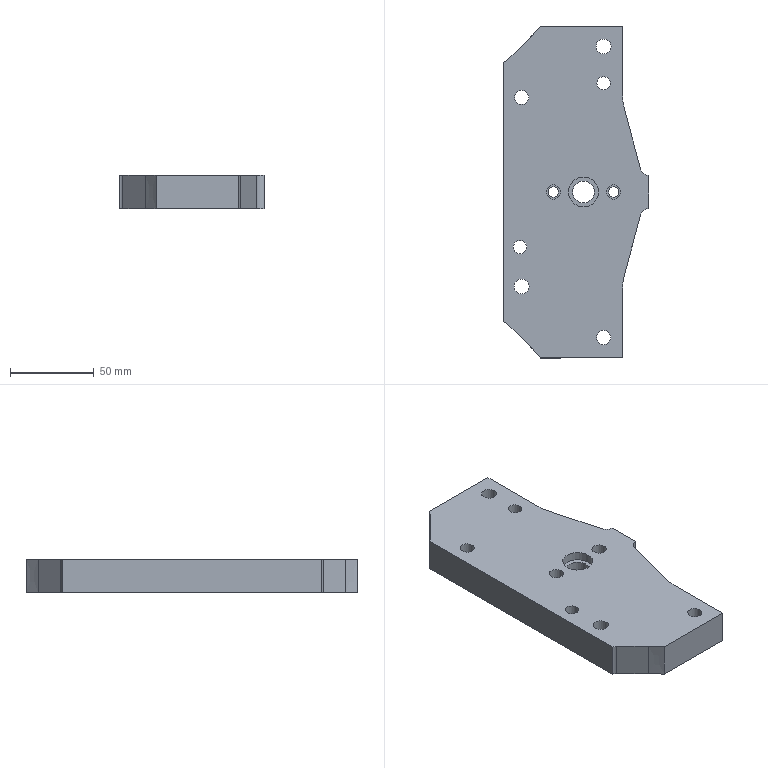Part | NX | features solid 2 | 1 solid | 47 faces | box 87 x 198.537 x 20 mm | volume 274052 mm3 | cylinder 24 | plane 21 | spline 2 | commonest cylinder face diameters 8.5 x6 8 x4 14 x4 6.1 x2 9 x2 10 x2
STEP:
#1=CARTESIAN_POINT('',(850.995,56.54,10.));
#2=VERTEX_POINT('',#1);
#3=CARTESIAN_POINT('',(843.995,56.54,10.));
#4=DIRECTION('',(0.,0.,-1.));
#5=DIRECTION('',(1.,0.,0.));
#6=AXIS2_PLACEMENT_3D('',#3,#4,#5);
#7=CIRCLE('',#6,7.);
#8=EDGE_CURVE('',#2,#2,#7,.T.);
#9=ORIENTED_EDGE('',*,*,#8,.F.);
#10=EDGE_LOOP('',(#9));
#11=FACE_BOUND('',#10,.T.);
#12=CARTESIAN_POINT('',(850.995,56.54,0.00000121));
#13=VERTEX_POINT('',#12);
#14=CARTESIAN_POINT('',(843.995,56.54,0.00000121));
#15=DIRECTION('',(0.,0.,-1.));
#16=DIRECTION('',(1.,0.,0.));
#17=AXIS2_PLACEMENT_3D('',#14,#15,#16);
#18=CIRCLE('',#17,7.);
#19=EDGE_CURVE('',#13,#13,#18,.F.);
#20=ORIENTED_EDGE('',*,*,#19,.F.);
#21=EDGE_LOOP('',(#20));
#22=FACE_BOUND('',#21,.T.);
#23=CARTESIAN_POINT('',(843.995,56.54,0.00000121));
#24=DIRECTION('',(0.,0.,1.));
#25=DIRECTION('',(1.,0.,0.));
#26=AXIS2_PLACEMENT_3D('',#23,#24,#25);
#27=CYLINDRICAL_SURFACE('',#26,7.);
#28=ADVANCED_FACE('',(#11,#22),#27,.F.);
#29=CARTESIAN_POINT('',(848.245,56.54,10.));
#30=VERTEX_POINT('',#29);
#31=CARTESIAN_POINT('',(843.995,56.54,10.));
#32=DIRECTION('',(0.,0.,-1.));
#33=DIRECTION('',(1.,0.,0.));
#34=AXIS2_PLACEMENT_3D('',#31,#32,#33);
#35=CIRCLE('',#34,4.25);
#36=EDGE_CURVE('',#30,#30,#35,.T.);
#37=ORIENTED_EDGE('',*,*,#36,.T.);
#38=EDGE_LOOP('',(#37));
#39=FACE_BOUND('',#38,.T.);
#40=CARTESIAN_POINT('',(839.745,56.54,20.));
#41=VERTEX_POINT('',#40);
#42=CARTESIAN_POINT('',(843.995,56.54,20.));
#43=DIRECTION('',(0.,0.,1.));
#44=DIRECTION('',(-1.,0.,0.));
#45=AXIS2_PLACEMENT_3D('',#42,#43,#44);
#46=CIRCLE('',#45,4.25);
#47=EDGE_CURVE('',#41,#41,#46,.F.);
#48=ORIENTED_EDGE('',*,*,#47,.F.);
#49=EDGE_LOOP('',(#48));
#50=FACE_BOUND('',#49,.T.);
#51=CARTESIAN_POINT('',(843.995,56.54,35.));
#52=DIRECTION('',(0.,0.,1.));
#53=DIRECTION('',(1.,0.,0.));
#54=AXIS2_PLACEMENT_3D('',#51,#52,#53);
#55=CYLINDRICAL_SURFACE('',#54,4.25);
#56=ADVANCED_FACE('',(#39,#50),#55,.F.);
#57=ORIENTED_EDGE('',*,*,#36,.F.);
#58=EDGE_LOOP('',(#57));
#59=FACE_BOUND('',#58,.T.);
#60=ORIENTED_EDGE('',*,*,#8,.T.);
#61=EDGE_LOOP('',(#60));
#62=FACE_BOUND('',#61,.T.);
#63=CARTESIAN_POINT('',(842.971,56.54,10.));
#64=DIRECTION('',(0.,0.,1.));
#65=DIRECTION('',(1.,0.,0.));
#66=AXIS2_PLACEMENT_3D('',#63,#64,#65);
#67=PLANE('',#66);
#68=ADVANCED_FACE('',(#59,#62),#67,.F.);
#69=CARTESIAN_POINT('',(897.245,-87.024,10.));
#70=VERTEX_POINT('',#69);
#71=CARTESIAN_POINT('',(892.995,-87.024,10.));
#72=DIRECTION('',(0.,0.,1.));
#73=DIRECTION('',(1.,0.,0.));
#74=AXIS2_PLACEMENT_3D('',#71,#72,#73);
#75=CIRCLE('',#74,4.25);
#76=EDGE_CURVE('',#70,#70,#75,.F.);
#77=ORIENTED_EDGE('',*,*,#76,.F.);
#78=EDGE_LOOP('',(#77));
#79=FACE_BOUND('',#78,.T.);
#80=CARTESIAN_POINT('',(899.995,-87.024,10.));
#81=VERTEX_POINT('',#80);
#82=CARTESIAN_POINT('',(892.995,-87.024,10.));
#83=DIRECTION('',(0.,0.,1.));
#84=DIRECTION('',(1.,0.,0.));
#85=AXIS2_PLACEMENT_3D('',#82,#83,#84);
#86=CIRCLE('',#85,7.);
#87=EDGE_CURVE('',#81,#81,#86,.F.);
#88=ORIENTED_EDGE('',*,*,#87,.T.);
#89=EDGE_LOOP('',(#88));
#90=FACE_BOUND('',#89,.T.);
#91=CARTESIAN_POINT('',(889.203,-87.719,10.));
#92=DIRECTION('',(0.,0.,1.));
#93=DIRECTION('',(1.,0.,0.));
#94=AXIS2_PLACEMENT_3D('',#91,#92,#93);
#95=PLANE('',#94);
#96=ADVANCED_FACE('',(#79,#90),#95,.F.);
#97=CARTESIAN_POINT('',(897.495,87.024,10.));
#98=VERTEX_POINT('',#97);
#99=CARTESIAN_POINT('',(892.995,87.024,10.));
#100=DIRECTION('',(0.,0.,1.));
#101=DIRECTION('',(1.,0.,0.));
#102=AXIS2_PLACEMENT_3D('',#99,#100,#101);
#103=CIRCLE('',#102,4.5);
#104=EDGE_CURVE('',#98,#98,#103,.F.);
#105=ORIENTED_EDGE('',*,*,#104,.F.);
#106=EDGE_LOOP('',(#105));
#107=FACE_BOUND('',#106,.T.);
#108=CARTESIAN_POINT('',(899.995,87.024,10.));
#109=VERTEX_POINT('',#108);
#110=CARTESIAN_POINT('',(892.995,87.024,10.));
#111=DIRECTION('',(0.,0.,-1.));
#112=DIRECTION('',(1.,0.,0.));
#113=AXIS2_PLACEMENT_3D('',#110,#111,#112);
#114=CIRCLE('',#113,7.);
#115=EDGE_CURVE('',#109,#109,#114,.T.);
#116=ORIENTED_EDGE('',*,*,#115,.T.);
#117=EDGE_LOOP('',(#116));
#118=FACE_BOUND('',#117,.T.);
#119=CARTESIAN_POINT('',(889.203,87.719,10.));
#120=DIRECTION('',(0.,0.,1.));
#121=DIRECTION('',(1.,0.,0.));
#122=AXIS2_PLACEMENT_3D('',#119,#120,#121);
#123=PLANE('',#122);
#124=ADVANCED_FACE('',(#107,#118),#123,.F.);
#125=CARTESIAN_POINT('',(848.495,-56.54,10.));
#126=VERTEX_POINT('',#125);
#127=CARTESIAN_POINT('',(843.995,-56.54,10.));
#128=DIRECTION('',(0.,0.,1.));
#129=DIRECTION('',(1.,0.,0.));
#130=AXIS2_PLACEMENT_3D('',#127,#128,#129);
#131=CIRCLE('',#130,4.5);
#132=EDGE_CURVE('',#126,#126,#131,.F.);
#133=ORIENTED_EDGE('',*,*,#132,.F.);
#134=EDGE_LOOP('',(#133));
#135=FACE_BOUND('',#134,.T.);
#136=CARTESIAN_POINT('',(850.995,-56.54,10.));
#137=VERTEX_POINT('',#136);
#138=CARTESIAN_POINT('',(843.995,-56.54,10.));
#139=DIRECTION('',(0.,0.,1.));
#140=DIRECTION('',(1.,0.,0.));
#141=AXIS2_PLACEMENT_3D('',#138,#139,#140);
#142=CIRCLE('',#141,7.);
#143=EDGE_CURVE('',#137,#137,#142,.F.);
#144=ORIENTED_EDGE('',*,*,#143,.T.);
#145=EDGE_LOOP('',(#144));
#146=FACE_BOUND('',#145,.T.);
#147=CARTESIAN_POINT('',(842.971,-56.54,10.));
#148=DIRECTION('',(0.,0.,1.));
#149=DIRECTION('',(1.,0.,0.));
#150=AXIS2_PLACEMENT_3D('',#147,#148,#149);
#151=PLANE('',#150);
#152=ADVANCED_FACE('',(#135,#146),#151,.F.);
#153=CARTESIAN_POINT('',(835.122,-78.661,20.));
#154=VERTEX_POINT('',#153);
#155=CARTESIAN_POINT('',(832.995,-77.568,20.));
#156=VERTEX_POINT('',#155);
#157=CARTESIAN_POINT('',(832.313,-81.509,20.));
#158=DIRECTION('',(0.,0.,-1.));
#159=DIRECTION('',(-1.,0.,0.));
#160=AXIS2_PLACEMENT_3D('',#157,#158,#159);
#161=CIRCLE('',#160,4.);
#162=EDGE_CURVE('',#154,#156,#161,.F.);
#163=ORIENTED_EDGE('',*,*,#162,.T.);
#164=CARTESIAN_POINT('',(832.995,-77.568,0.00000121));
#165=VERTEX_POINT('',#164);
#166=CARTESIAN_POINT('',(832.995,-77.568,108.));
#167=DIRECTION('',(0.,0.,1.));
#168=VECTOR('',#167,1000.);
#169=LINE('',#166,#168);
#170=EDGE_CURVE('',#156,#165,#169,.F.);
#171=ORIENTED_EDGE('',*,*,#170,.T.);
#172=CARTESIAN_POINT('',(835.122,-78.661,0.00000121));
#173=VERTEX_POINT('',#172);
#174=CARTESIAN_POINT('',(832.313,-81.509,0.00000121));
#175=DIRECTION('',(0.,0.,-1.));
#176=DIRECTION('',(-1.,0.,0.));
#177=AXIS2_PLACEMENT_3D('',#174,#175,#176);
#178=CIRCLE('',#177,4.);
#179=EDGE_CURVE('',#173,#165,#178,.F.);
#180=ORIENTED_EDGE('',*,*,#179,.F.);
#181=CARTESIAN_POINT('',(835.122,-78.661,0.00000121));
#182=DIRECTION('',(0.,0.,-1.));
#183=VECTOR('',#182,1000.);
#184=LINE('',#181,#183);
#185=EDGE_CURVE('',#154,#173,#184,.T.);
#186=ORIENTED_EDGE('',*,*,#185,.F.);
#187=EDGE_LOOP('',(#163,#171,#180,#186));
#188=FACE_BOUND('',#187,.T.);
#189=CARTESIAN_POINT('',(832.313,-81.509,108.));
#190=DIRECTION('',(0.,0.,1.));
#191=DIRECTION('',(1.,0.,0.));
#192=AXIS2_PLACEMENT_3D('',#189,#190,#191);
#193=CYLINDRICAL_SURFACE('',#192,4.);
#194=ADVANCED_FACE('',(#188),#193,.F.);
#195=ORIENTED_EDGE('',*,*,#170,.F.);
#196=CARTESIAN_POINT('',(832.995,77.568,20.));
#197=VERTEX_POINT('',#196);
#198=CARTESIAN_POINT('',(832.995,97.031,20.));
#199=DIRECTION('',(0.,1.,0.));
#200=VECTOR('',#199,1000.);
#201=LINE('',#198,#200);
#202=EDGE_CURVE('',#156,#197,#201,.T.);
#203=ORIENTED_EDGE('',*,*,#202,.T.);
#204=CARTESIAN_POINT('',(832.995,77.568,0.00000121));
#205=VERTEX_POINT('',#204);
#206=CARTESIAN_POINT('',(832.995,77.568,108.));
#207=DIRECTION('',(0.,0.,1.));
#208=VECTOR('',#207,1000.);
#209=LINE('',#206,#208);
#210=EDGE_CURVE('',#205,#197,#209,.T.);
#211=ORIENTED_EDGE('',*,*,#210,.F.);
#212=CARTESIAN_POINT('',(832.995,0.,0.00000121));
#213=DIRECTION('',(0.,1.,0.));
#214=VECTOR('',#213,1000.);
#215=LINE('',#212,#214);
#216=EDGE_CURVE('',#165,#205,#215,.T.);
#217=ORIENTED_EDGE('',*,*,#216,.F.);
#218=EDGE_LOOP('',(#195,#203,#211,#217));
#219=FACE_BOUND('',#218,.T.);
#220=CARTESIAN_POINT('',(832.995,97.031,20.));
#221=DIRECTION('',(-1.,0.,0.));
#222=DIRECTION('',(0.,1.,0.));
#223=AXIS2_PLACEMENT_3D('',#220,#221,#222);
#224=PLANE('',#223);
#225=ADVANCED_FACE('',(#219),#224,.T.);
#226=CARTESIAN_POINT('',(835.122,78.661,0.00000121));
#227=VERTEX_POINT('',#226);
#228=CARTESIAN_POINT('',(832.313,81.509,0.00000121));
#229=DIRECTION('',(0.,0.,-1.));
#230=DIRECTION('',(-1.,0.,0.));
#231=AXIS2_PLACEMENT_3D('',#228,#229,#230);
#232=CIRCLE('',#231,4.);
#233=EDGE_CURVE('',#205,#227,#232,.F.);
#234=ORIENTED_EDGE('',*,*,#233,.F.);
#235=ORIENTED_EDGE('',*,*,#210,.T.);
#236=CARTESIAN_POINT('',(835.122,78.661,20.));
#237=VERTEX_POINT('',#236);
#238=CARTESIAN_POINT('',(832.313,81.509,20.));
#239=DIRECTION('',(0.,0.,-1.));
#240=DIRECTION('',(-1.,0.,0.));
#241=AXIS2_PLACEMENT_3D('',#238,#239,#240);
#242=CIRCLE('',#241,4.);
#243=EDGE_CURVE('',#197,#237,#242,.F.);
#244=ORIENTED_EDGE('',*,*,#243,.T.);
#245=CARTESIAN_POINT('',(835.122,78.661,0.00000121));
#246=DIRECTION('',(0.,0.,-1.));
#247=VECTOR('',#246,1000.);
#248=LINE('',#245,#247);
#249=EDGE_CURVE('',#227,#237,#248,.F.);
#250=ORIENTED_EDGE('',*,*,#249,.F.);
#251=EDGE_LOOP('',(#234,#235,#244,#250));
#252=FACE_BOUND('',#251,.T.);
#253=CARTESIAN_POINT('',(832.313,81.509,108.));
#254=DIRECTION('',(0.,0.,1.));
#255=DIRECTION('',(1.,0.,0.));
#256=AXIS2_PLACEMENT_3D('',#253,#254,#255);
#257=CYLINDRICAL_SURFACE('',#256,4.);
#258=ADVANCED_FACE('',(#252),#257,.F.);
#259=CARTESIAN_POINT('',(848.684,92.039,20.));
#260=VERTEX_POINT('',#259);
#261=CARTESIAN_POINT('',(837.389,80.898,20.));
#262=DIRECTION('',(-0.7119,-0.7022,0.));
#263=VECTOR('',#262,1000.);
#264=LINE('',#261,#263);
#265=EDGE_CURVE('',#260,#237,#264,.T.);
#266=ORIENTED_EDGE('',*,*,#265,.F.);
#267=CARTESIAN_POINT('',(848.684,92.039,0.00000121));
#268=VERTEX_POINT('',#267);
#269=CARTESIAN_POINT('',(848.684,92.039,0.00000121));
#270=CARTESIAN_POINT('',(848.684,92.039,6.667));
#271=CARTESIAN_POINT('',(848.684,92.039,13.333));
#272=CARTESIAN_POINT('',(848.684,92.039,20.));
#273=B_SPLINE_CURVE_WITH_KNOTS('',3,(#269,#270,#271,#272),.UNSPECIFIED.,.F.,.F.,(4,4),(0.5581,0.6662),.UNSPECIFIED.);
#274=EDGE_CURVE('',#260,#268,#273,.F.);
#275=ORIENTED_EDGE('',*,*,#274,.T.);
#276=CARTESIAN_POINT('',(654.957,-99.049,0.00000121));
#277=DIRECTION('',(0.7119,0.7022,0.));
#278=VECTOR('',#277,1000.);
#279=LINE('',#276,#278);
#280=EDGE_CURVE('',#268,#227,#279,.F.);
#281=ORIENTED_EDGE('',*,*,#280,.T.);
#282=ORIENTED_EDGE('',*,*,#249,.T.);
#283=EDGE_LOOP('',(#266,#275,#281,#282));
#284=FACE_BOUND('',#283,.T.);
#285=CARTESIAN_POINT('',(837.389,80.898,36.75));
#286=DIRECTION('',(-0.7022,0.7119,0.));
#287=DIRECTION('',(-0.7119,-0.7022,0.));
#288=AXIS2_PLACEMENT_3D('',#285,#286,#287);
#289=PLANE('',#288);
#290=ADVANCED_FACE('',(#284),#289,.T.);
#291=CARTESIAN_POINT('',(855.037,99.269,0.00000121));
#292=VERTEX_POINT('',#291);
#293=CARTESIAN_POINT('',(855.037,99.269,20.));
#294=VERTEX_POINT('',#293);
#295=CARTESIAN_POINT('',(855.037,99.269,0.00000121));
#296=DIRECTION('',(0.,0.,-1.));
#297=VECTOR('',#296,1000.);
#298=LINE('',#295,#297);
#299=EDGE_CURVE('',#292,#294,#298,.F.);
#300=ORIENTED_EDGE('',*,*,#299,.F.);
#301=CARTESIAN_POINT('',(855.037,99.269,0.00000121));
#302=CARTESIAN_POINT('',(853.124,96.673,0.00000121));
#303=CARTESIAN_POINT('',(850.954,94.278,0.00000121));
#304=CARTESIAN_POINT('',(848.684,92.039,0.00000121));
#305=B_SPLINE_CURVE_WITH_KNOTS('',3,(#301,#302,#303,#304),.UNSPECIFIED.,.F.,.F.,(4,4),(0.01581,0.02521),.UNSPECIFIED.);
#306=EDGE_CURVE('',#292,#268,#305,.T.);
#307=ORIENTED_EDGE('',*,*,#306,.T.);
#308=ORIENTED_EDGE('',*,*,#274,.F.);
#309=CARTESIAN_POINT('',(855.037,99.269,20.));
#310=CARTESIAN_POINT('',(853.129,96.679,20.));
#311=CARTESIAN_POINT('',(850.976,94.3,20.));
#312=CARTESIAN_POINT('',(848.684,92.039,20.));
#313=B_SPLINE_CURVE_WITH_KNOTS('',3,(#309,#310,#311,#312),.UNSPECIFIED.,.F.,.F.,(4,4),(0.001457,0.01108),.UNSPECIFIED.);
#314=EDGE_CURVE('',#294,#260,#313,.T.);
#315=ORIENTED_EDGE('',*,*,#314,.F.);
#316=EDGE_LOOP('',(#300,#307,#308,#315));
#317=FACE_BOUND('',#316,.T.);
#318=CARTESIAN_POINT('',(855.037,99.269,20.));
#319=CARTESIAN_POINT('',(853.124,96.673,20.));
#320=CARTESIAN_POINT('',(850.954,94.279,20.));
#321=CARTESIAN_POINT('',(848.684,92.039,20.));
#322=CARTESIAN_POINT('',(855.037,99.269,13.333));
#323=CARTESIAN_POINT('',(853.124,96.673,13.333));
#324=CARTESIAN_POINT('',(850.954,94.279,13.333));
#325=CARTESIAN_POINT('',(848.684,92.039,13.333));
#326=CARTESIAN_POINT('',(855.037,99.269,6.667));
#327=CARTESIAN_POINT('',(853.124,96.673,6.667));
#328=CARTESIAN_POINT('',(850.954,94.279,6.667));
#329=CARTESIAN_POINT('',(848.684,92.039,6.667));
#330=CARTESIAN_POINT('',(855.037,99.269,0.00000121));
#331=CARTESIAN_POINT('',(853.124,96.673,0.00000121));
#332=CARTESIAN_POINT('',(850.954,94.279,0.00000121));
#333=CARTESIAN_POINT('',(848.684,92.039,0.00000121));
#334=B_SPLINE_SURFACE_WITH_KNOTS('',3,3,((#318,#319,#320,#321),(#322,#323,#324,#325),(#326,#327,#328,#329),(#330,#331,#332,#333)),.UNSPECIFIED.,.F.,.F.,.F.,(4,4),(4,4),(0.3338,0.4419),(0.01581,0.02521),.UNSPECIFIED.);
#335=ADVANCED_FACE('',(#317),#334,.T.);
#336=CARTESIAN_POINT('',(904.337,99.269,0.00000121));
#337=VERTEX_POINT('',#336);
#338=CARTESIAN_POINT('',(559.023,99.269,0.00000121));
#339=DIRECTION('',(1.,0.,0.));
#340=VECTOR('',#339,1000.);
#341=LINE('',#338,#340);
#342=EDGE_CURVE('',#292,#337,#341,.T.);
#343=ORIENTED_EDGE('',*,*,#342,.F.);
#344=ORIENTED_EDGE('',*,*,#299,.T.);
#345=CARTESIAN_POINT('',(904.337,99.269,20.));
#346=VERTEX_POINT('',#345);
#347=CARTESIAN_POINT('',(893.317,99.269,20.));
#348=DIRECTION('',(1.,0.,0.));
#349=VECTOR('',#348,1000.);
#350=LINE('',#347,#349);
#351=EDGE_CURVE('',#294,#346,#350,.T.);
#352=ORIENTED_EDGE('',*,*,#351,.T.);
#353=CARTESIAN_POINT('',(904.337,99.269,20.));
#354=DIRECTION('',(0.,0.,-1.));
#355=VECTOR('',#354,1000.);
#356=LINE('',#353,#355);
#357=EDGE_CURVE('',#337,#346,#356,.F.);
#358=ORIENTED_EDGE('',*,*,#357,.F.);
#359=EDGE_LOOP('',(#343,#344,#352,#358));
#360=FACE_BOUND('',#359,.T.);
#361=CARTESIAN_POINT('',(893.317,99.269,20.));
#362=DIRECTION('',(0.,1.,0.));
#363=DIRECTION('',(1.,0.,0.));
#364=AXIS2_PLACEMENT_3D('',#361,#362,#363);
#365=PLANE('',#364);
#366=ADVANCED_FACE('',(#360),#365,.T.);
#367=CARTESIAN_POINT('',(904.337,57.474,0.00000121));
#368=VERTEX_POINT('',#367);
#369=CARTESIAN_POINT('',(904.337,-6.048,0.00000121));
#370=DIRECTION('',(0.,-1.,0.));
#371=VECTOR('',#370,1000.);
#372=LINE('',#369,#371);
#373=EDGE_CURVE('',#368,#337,#372,.F.);
#374=ORIENTED_EDGE('',*,*,#373,.T.);
#375=ORIENTED_EDGE('',*,*,#357,.T.);
#376=CARTESIAN_POINT('',(904.337,57.474,20.));
#377=VERTEX_POINT('',#376);
#378=CARTESIAN_POINT('',(904.337,136.981,20.));
#379=DIRECTION('',(0.,1.,0.));
#380=VECTOR('',#379,1000.);
#381=LINE('',#378,#380);
#382=EDGE_CURVE('',#377,#346,#381,.T.);
#383=ORIENTED_EDGE('',*,*,#382,.F.);
#384=CARTESIAN_POINT('',(904.337,57.473,-160.));
#385=DIRECTION('',(0.,0.,1.));
#386=VECTOR('',#385,1000.);
#387=LINE('',#384,#386);
#388=EDGE_CURVE('',#368,#377,#387,.T.);
#389=ORIENTED_EDGE('',*,*,#388,.F.);
#390=EDGE_LOOP('',(#374,#375,#383,#389));
#391=FACE_BOUND('',#390,.T.);
#392=CARTESIAN_POINT('',(904.337,136.981,-160.));
#393=DIRECTION('',(1.,0.,0.));
#394=DIRECTION('',(0.,-1.,0.));
#395=AXIS2_PLACEMENT_3D('',#392,#393,#394);
#396=PLANE('',#395);
#397=ADVANCED_FACE('',(#391),#396,.T.);
#398=CARTESIAN_POINT('',(905.257,50.485,20.));
#399=VERTEX_POINT('',#398);
#400=CARTESIAN_POINT('',(931.337,57.473,20.));
#401=DIRECTION('',(0.,0.,-1.));
#402=DIRECTION('',(-1.,0.,0.));
#403=AXIS2_PLACEMENT_3D('',#400,#401,#402);
#404=CIRCLE('',#403,27.);
#405=EDGE_CURVE('',#399,#377,#404,.T.);
#406=ORIENTED_EDGE('',*,*,#405,.F.);
#407=CARTESIAN_POINT('',(905.257,50.485,0.00000121));
#408=VERTEX_POINT('',#407);
#409=CARTESIAN_POINT('',(905.257,50.485,-160.));
#410=DIRECTION('',(0.,0.,1.));
#411=VECTOR('',#410,1000.);
#412=LINE('',#409,#411);
#413=EDGE_CURVE('',#408,#399,#412,.T.);
#414=ORIENTED_EDGE('',*,*,#413,.F.);
#415=CARTESIAN_POINT('',(931.337,57.473,0.00000121));
#416=DIRECTION('',(0.,0.,-1.));
#417=DIRECTION('',(-1.,0.,0.));
#418=AXIS2_PLACEMENT_3D('',#415,#416,#417);
#419=CIRCLE('',#418,27.);
#420=EDGE_CURVE('',#408,#368,#419,.T.);
#421=ORIENTED_EDGE('',*,*,#420,.T.);
#422=ORIENTED_EDGE('',*,*,#388,.T.);
#423=EDGE_LOOP('',(#406,#414,#421,#422));
#424=FACE_BOUND('',#423,.T.);
#425=CARTESIAN_POINT('',(931.337,57.473,-160.));
#426=DIRECTION('',(0.,0.,1.));
#427=DIRECTION('',(1.,0.,0.));
#428=AXIS2_PLACEMENT_3D('',#425,#426,#427);
#429=CYLINDRICAL_SURFACE('',#428,27.);
#430=ADVANCED_FACE('',(#424),#429,.F.);
#431=CARTESIAN_POINT('',(915.166,13.504,20.));
#432=VERTEX_POINT('',#431);
#433=CARTESIAN_POINT('',(904.576,53.027,20.));
#434=DIRECTION('',(-0.2588,0.9659,0.));
#435=VECTOR('',#434,1000.);
#436=LINE('',#433,#435);
#437=EDGE_CURVE('',#432,#399,#436,.T.);
#438=ORIENTED_EDGE('',*,*,#437,.F.);
#439=CARTESIAN_POINT('',(915.166,13.504,0.00000121));
#440=VERTEX_POINT('',#439);
#441=CARTESIAN_POINT('',(915.166,13.504,-160.));
#442=DIRECTION('',(0.,0.,1.));
#443=VECTOR('',#442,1000.);
#444=LINE('',#441,#443);
#445=EDGE_CURVE('',#440,#432,#444,.T.);
#446=ORIENTED_EDGE('',*,*,#445,.F.);
#447=CARTESIAN_POINT('',(894.567,90.382,0.00000121));
#448=DIRECTION('',(0.2588,-0.9659,0.));
#449=VECTOR('',#448,1000.);
#450=LINE('',#447,#449);
#451=EDGE_CURVE('',#440,#408,#450,.F.);
#452=ORIENTED_EDGE('',*,*,#451,.T.);
#453=ORIENTED_EDGE('',*,*,#413,.T.);
#454=EDGE_LOOP('',(#438,#446,#452,#453));
#455=FACE_BOUND('',#454,.T.);
#456=CARTESIAN_POINT('',(904.576,53.027,-160.));
#457=DIRECTION('',(0.9659,0.2588,0.));
#458=DIRECTION('',(0.2588,-0.9659,0.));
#459=AXIS2_PLACEMENT_3D('',#456,#457,#458);
#460=PLANE('',#459);
#461=ADVANCED_FACE('',(#455),#460,.T.);
#462=CARTESIAN_POINT('',(919.996,9.798,20.));
#463=VERTEX_POINT('',#462);
#464=CARTESIAN_POINT('',(919.996,14.798,20.));
#465=DIRECTION('',(0.,0.,-1.));
#466=DIRECTION('',(-1.,0.,0.));
#467=AXIS2_PLACEMENT_3D('',#464,#465,#466);
#468=CIRCLE('',#467,5.);
#469=EDGE_CURVE('',#463,#432,#468,.T.);
#470=ORIENTED_EDGE('',*,*,#469,.F.);
#471=CARTESIAN_POINT('',(919.996,9.798,0.00000121));
#472=VERTEX_POINT('',#471);
#473=CARTESIAN_POINT('',(919.996,9.798,20.));
#474=DIRECTION('',(0.,0.,-1.));
#475=VECTOR('',#474,1000.);
#476=LINE('',#473,#475);
#477=EDGE_CURVE('',#472,#463,#476,.F.);
#478=ORIENTED_EDGE('',*,*,#477,.F.);
#479=CARTESIAN_POINT('',(919.996,14.798,0.00000121));
#480=DIRECTION('',(0.,0.,-1.));
#481=DIRECTION('',(-1.,0.,0.));
#482=AXIS2_PLACEMENT_3D('',#479,#480,#481);
#483=CIRCLE('',#482,5.);
#484=EDGE_CURVE('',#472,#440,#483,.T.);
#485=ORIENTED_EDGE('',*,*,#484,.T.);
#486=ORIENTED_EDGE('',*,*,#445,.T.);
#487=EDGE_LOOP('',(#470,#478,#485,#486));
#488=FACE_BOUND('',#487,.T.);
#489=CARTESIAN_POINT('',(919.996,14.798,-160.));
#490=DIRECTION('',(0.,0.,1.));
#491=DIRECTION('',(1.,0.,0.));
#492=AXIS2_PLACEMENT_3D('',#489,#490,#491);
#493=CYLINDRICAL_SURFACE('',#492,5.);
#494=ADVANCED_FACE('',(#488),#493,.F.);
#495=CARTESIAN_POINT('',(919.996,-9.798,0.00000121));
#496=VERTEX_POINT('',#495);
#497=CARTESIAN_POINT('',(919.996,0.,0.00000121));
#498=DIRECTION('',(0.,-1.,0.));
#499=VECTOR('',#498,1000.);
#500=LINE('',#497,#499);
#501=EDGE_CURVE('',#472,#496,#500,.T.);
#502=ORIENTED_EDGE('',*,*,#501,.F.);
#503=ORIENTED_EDGE('',*,*,#477,.T.);
#504=CARTESIAN_POINT('',(919.996,-9.798,20.));
#505=VERTEX_POINT('',#504);
#506=CARTESIAN_POINT('',(919.996,-14.798,20.));
#507=DIRECTION('',(0.,-1.,0.));
#508=VECTOR('',#507,1000.);
#509=LINE('',#506,#508);
#510=EDGE_CURVE('',#463,#505,#509,.T.);
#511=ORIENTED_EDGE('',*,*,#510,.T.);
#512=CARTESIAN_POINT('',(919.996,-9.798,20.));
#513=DIRECTION('',(0.,0.,-1.));
#514=VECTOR('',#513,1000.);
#515=LINE('',#512,#514);
#516=EDGE_CURVE('',#496,#505,#515,.F.);
#517=ORIENTED_EDGE('',*,*,#516,.F.);
#518=EDGE_LOOP('',(#502,#503,#511,#517));
#519=FACE_BOUND('',#518,.T.);
#520=CARTESIAN_POINT('',(919.996,-14.798,20.));
#521=DIRECTION('',(1.,0.,0.));
#522=DIRECTION('',(0.,-1.,0.));
#523=AXIS2_PLACEMENT_3D('',#520,#521,#522);
#524=PLANE('',#523);
#525=ADVANCED_FACE('',(#519),#524,.T.);
#526=CARTESIAN_POINT('',(915.166,-13.504,0.00000121));
#527=VERTEX_POINT('',#526);
#528=CARTESIAN_POINT('',(919.996,-14.798,0.00000121));
#529=DIRECTION('',(0.,0.,-1.));
#530=DIRECTION('',(-1.,0.,0.));
#531=AXIS2_PLACEMENT_3D('',#528,#529,#530);
#532=CIRCLE('',#531,5.);
#533=EDGE_CURVE('',#496,#527,#532,.F.);
#534=ORIENTED_EDGE('',*,*,#533,.F.);
#535=ORIENTED_EDGE('',*,*,#516,.T.);
#536=CARTESIAN_POINT('',(915.166,-13.504,20.));
#537=VERTEX_POINT('',#536);
#538=CARTESIAN_POINT('',(919.996,-14.798,20.));
#539=DIRECTION('',(0.,0.,-1.));
#540=DIRECTION('',(-1.,0.,0.));
#541=AXIS2_PLACEMENT_3D('',#538,#539,#540);
#542=CIRCLE('',#541,5.);
#543=EDGE_CURVE('',#505,#537,#542,.F.);
#544=ORIENTED_EDGE('',*,*,#543,.T.);
#545=CARTESIAN_POINT('',(915.166,-13.504,40.));
#546=DIRECTION('',(0.,0.,-1.));
#547=VECTOR('',#546,1000.);
#548=LINE('',#545,#547);
#549=EDGE_CURVE('',#527,#537,#548,.F.);
#550=ORIENTED_EDGE('',*,*,#549,.F.);
#551=EDGE_LOOP('',(#534,#535,#544,#550));
#552=FACE_BOUND('',#551,.T.);
#553=CARTESIAN_POINT('',(919.996,-14.798,82.75));
#554=DIRECTION('',(0.,0.,1.));
#555=DIRECTION('',(1.,0.,0.));
#556=AXIS2_PLACEMENT_3D('',#553,#554,#555);
#557=CYLINDRICAL_SURFACE('',#556,5.);
#558=ADVANCED_FACE('',(#552),#557,.F.);
#559=ORIENTED_EDGE('',*,*,#549,.T.);
#560=CARTESIAN_POINT('',(905.257,-50.485,20.));
#561=VERTEX_POINT('',#560);
#562=CARTESIAN_POINT('',(904.576,-53.027,20.));
#563=DIRECTION('',(-0.2588,-0.9659,0.));
#564=VECTOR('',#563,1000.);
#565=LINE('',#562,#564);
#566=EDGE_CURVE('',#537,#561,#565,.T.);
#567=ORIENTED_EDGE('',*,*,#566,.T.);
#568=CARTESIAN_POINT('',(905.257,-50.485,0.00000121));
#569=VERTEX_POINT('',#568);
#570=CARTESIAN_POINT('',(905.257,-50.485,82.75));
#571=DIRECTION('',(0.,0.,-1.));
#572=VECTOR('',#571,1000.);
#573=LINE('',#570,#572);
#574=EDGE_CURVE('',#569,#561,#573,.F.);
#575=ORIENTED_EDGE('',*,*,#574,.F.);
#576=CARTESIAN_POINT('',(894.567,-90.382,0.00000121));
#577=DIRECTION('',(-0.2588,-0.9659,0.));
#578=VECTOR('',#577,1000.);
#579=LINE('',#576,#578);
#580=EDGE_CURVE('',#569,#527,#579,.F.);
#581=ORIENTED_EDGE('',*,*,#580,.T.);
#582=EDGE_LOOP('',(#559,#567,#575,#581));
#583=FACE_BOUND('',#582,.T.);
#584=CARTESIAN_POINT('',(929.971,41.749,82.75));
#585=DIRECTION('',(0.9659,-0.2588,0.));
#586=DIRECTION('',(-0.2588,-0.9659,0.));
#587=AXIS2_PLACEMENT_3D('',#584,#585,#586);
#588=PLANE('',#587);
#589=ADVANCED_FACE('',(#583),#588,.T.);
#590=ORIENTED_EDGE('',*,*,#574,.T.);
#591=CARTESIAN_POINT('',(904.337,-57.474,20.));
#592=VERTEX_POINT('',#591);
#593=CARTESIAN_POINT('',(931.337,-57.473,20.));
#594=DIRECTION('',(0.,0.,-1.));
#595=DIRECTION('',(-1.,0.,0.));
#596=AXIS2_PLACEMENT_3D('',#593,#594,#595);
#597=CIRCLE('',#596,27.);
#598=EDGE_CURVE('',#561,#592,#597,.F.);
#599=ORIENTED_EDGE('',*,*,#598,.T.);
#600=CARTESIAN_POINT('',(904.337,-57.474,0.00000121));
#601=VERTEX_POINT('',#600);
#602=CARTESIAN_POINT('',(904.337,-57.473,82.75));
#603=DIRECTION('',(0.,0.,1.));
#604=VECTOR('',#603,1000.);
#605=LINE('',#602,#604);
#606=EDGE_CURVE('',#601,#592,#605,.T.);
#607=ORIENTED_EDGE('',*,*,#606,.F.);
#608=CARTESIAN_POINT('',(931.337,-57.473,0.00000121));
#609=DIRECTION('',(0.,0.,-1.));
#610=DIRECTION('',(-1.,0.,0.));
#611=AXIS2_PLACEMENT_3D('',#608,#609,#610);
#612=CIRCLE('',#611,27.);
#613=EDGE_CURVE('',#601,#569,#612,.T.);
#614=ORIENTED_EDGE('',*,*,#613,.T.);
#615=EDGE_LOOP('',(#590,#599,#607,#614));
#616=FACE_BOUND('',#615,.T.);
#617=CARTESIAN_POINT('',(931.337,-57.473,82.75));
#618=DIRECTION('',(0.,0.,-1.));
#619=DIRECTION('',(-1.,0.,0.));
#620=AXIS2_PLACEMENT_3D('',#617,#618,#619);
#621=CYLINDRICAL_SURFACE('',#620,27.);
#622=ADVANCED_FACE('',(#616),#621,.F.);
#623=ORIENTED_EDGE('',*,*,#606,.T.);
#624=CARTESIAN_POINT('',(904.337,-99.269,20.));
#625=VERTEX_POINT('',#624);
#626=CARTESIAN_POINT('',(904.337,-137.007,20.));
#627=DIRECTION('',(0.,-1.,0.));
#628=VECTOR('',#627,1000.);
#629=LINE('',#626,#628);
#630=EDGE_CURVE('',#592,#625,#629,.T.);
#631=ORIENTED_EDGE('',*,*,#630,.T.);
#632=CARTESIAN_POINT('',(904.337,-99.269,0.00000121));
#633=VERTEX_POINT('',#632);
#634=CARTESIAN_POINT('',(904.337,-99.269,82.75));
#635=DIRECTION('',(0.,0.,-1.));
#636=VECTOR('',#635,1000.);
#637=LINE('',#634,#636);
#638=EDGE_CURVE('',#633,#625,#637,.F.);
#639=ORIENTED_EDGE('',*,*,#638,.F.);
#640=CARTESIAN_POINT('',(904.337,6.022,0.00000121));
#641=DIRECTION('',(0.,-1.,0.));
#642=VECTOR('',#641,1000.);
#643=LINE('',#640,#642);
#644=EDGE_CURVE('',#633,#601,#643,.F.);
#645=ORIENTED_EDGE('',*,*,#644,.T.);
#646=EDGE_LOOP('',(#623,#631,#639,#645));
#647=FACE_BOUND('',#646,.T.);
#648=CARTESIAN_POINT('',(904.337,34.851,82.75));
#649=DIRECTION('',(1.,0.,0.));
#650=DIRECTION('',(0.,-1.,0.));
#651=AXIS2_PLACEMENT_3D('',#648,#649,#650);
#652=PLANE('',#651);
#653=ADVANCED_FACE('',(#647),#652,.T.);
#654=CARTESIAN_POINT('',(855.037,-99.269,20.));
#655=VERTEX_POINT('',#654);
#656=CARTESIAN_POINT('',(872.293,-99.269,20.));
#657=DIRECTION('',(-1.,0.,0.));
#658=VECTOR('',#657,1000.);
#659=LINE('',#656,#658);
#660=EDGE_CURVE('',#625,#655,#659,.T.);
#661=ORIENTED_EDGE('',*,*,#660,.T.);
#662=CARTESIAN_POINT('',(855.037,-99.269,0.00000121));
#663=VERTEX_POINT('',#662);
#664=CARTESIAN_POINT('',(855.037,-99.269,20.));
#665=DIRECTION('',(0.,0.,-1.));
#666=VECTOR('',#665,1000.);
#667=LINE('',#664,#666);
#668=EDGE_CURVE('',#655,#663,#667,.T.);
#669=ORIENTED_EDGE('',*,*,#668,.T.);
#670=CARTESIAN_POINT('',(559.026,-99.269,0.00000121));
#671=DIRECTION('',(-1.,0.,0.));
#672=VECTOR('',#671,1000.);
#673=LINE('',#670,#672);
#674=EDGE_CURVE('',#633,#663,#673,.T.);
#675=ORIENTED_EDGE('',*,*,#674,.F.);
#676=ORIENTED_EDGE('',*,*,#638,.T.);
#677=EDGE_LOOP('',(#661,#669,#675,#676));
#678=FACE_BOUND('',#677,.T.);
#679=CARTESIAN_POINT('',(872.293,-99.269,20.));
#680=DIRECTION('',(0.,-1.,0.));
#681=DIRECTION('',(-1.,0.,0.));
#682=AXIS2_PLACEMENT_3D('',#679,#680,#681);
#683=PLANE('',#682);
#684=ADVANCED_FACE('',(#678),#683,.T.);
#685=ORIENTED_EDGE('',*,*,#668,.F.);
#686=CARTESIAN_POINT('',(848.684,-92.039,20.));
#687=VERTEX_POINT('',#686);
#688=CARTESIAN_POINT('',(848.684,-92.039,20.));
#689=CARTESIAN_POINT('',(850.976,-94.3,20.));
#690=CARTESIAN_POINT('',(853.129,-96.679,20.));
#691=CARTESIAN_POINT('',(855.037,-99.269,20.));
#692=B_SPLINE_CURVE_WITH_KNOTS('',3,(#688,#689,#690,#691),.UNSPECIFIED.,.F.,.F.,(4,4),(0.,0.009624),.UNSPECIFIED.);
#693=EDGE_CURVE('',#687,#655,#692,.T.);
#694=ORIENTED_EDGE('',*,*,#693,.F.);
#695=CARTESIAN_POINT('',(848.684,-92.039,0.00000121));
#696=VERTEX_POINT('',#695);
#697=CARTESIAN_POINT('',(848.684,-92.039,0.00000121));
#698=CARTESIAN_POINT('',(848.684,-92.039,6.667));
#699=CARTESIAN_POINT('',(848.684,-92.039,13.333));
#700=CARTESIAN_POINT('',(848.684,-92.039,20.));
#701=B_SPLINE_CURVE_WITH_KNOTS('',3,(#697,#698,#699,#700),.UNSPECIFIED.,.F.,.F.,(4,4),(0.5581,0.6662),.UNSPECIFIED.);
#702=EDGE_CURVE('',#696,#687,#701,.T.);
#703=ORIENTED_EDGE('',*,*,#702,.F.);
#704=CARTESIAN_POINT('',(848.684,-92.039,0.00000121));
#705=CARTESIAN_POINT('',(850.972,-94.296,0.00000121));
#706=CARTESIAN_POINT('',(853.134,-96.686,0.00000121));
#707=CARTESIAN_POINT('',(855.037,-99.269,0.00000121));
#708=B_SPLINE_CURVE_WITH_KNOTS('',3,(#704,#705,#706,#707),.UNSPECIFIED.,.F.,.F.,(4,4),(0.,0.009632),.UNSPECIFIED.);
#709=EDGE_CURVE('',#696,#663,#708,.T.);
#710=ORIENTED_EDGE('',*,*,#709,.T.);
#711=EDGE_LOOP('',(#685,#694,#703,#710));
#712=FACE_BOUND('',#711,.T.);
#713=CARTESIAN_POINT('',(855.037,-99.269,20.));
#714=CARTESIAN_POINT('',(853.124,-96.673,20.));
#715=CARTESIAN_POINT('',(850.954,-94.279,20.));
#716=CARTESIAN_POINT('',(848.684,-92.039,20.));
#717=CARTESIAN_POINT('',(855.037,-99.269,13.333));
#718=CARTESIAN_POINT('',(853.124,-96.673,13.333));
#719=CARTESIAN_POINT('',(850.954,-94.279,13.333));
#720=CARTESIAN_POINT('',(848.684,-92.039,13.333));
#721=CARTESIAN_POINT('',(855.037,-99.269,6.667));
#722=CARTESIAN_POINT('',(853.124,-96.673,6.667));
#723=CARTESIAN_POINT('',(850.954,-94.279,6.667));
#724=CARTESIAN_POINT('',(848.684,-92.039,6.667));
#725=CARTESIAN_POINT('',(855.037,-99.269,0.00000121));
#726=CARTESIAN_POINT('',(853.124,-96.673,0.00000121));
#727=CARTESIAN_POINT('',(850.954,-94.279,0.00000121));
#728=CARTESIAN_POINT('',(848.684,-92.039,0.00000121));
#729=B_SPLINE_SURFACE_WITH_KNOTS('',3,3,((#713,#714,#715,#716),(#717,#718,#719,#720),(#721,#722,#723,#724),(#725,#726,#727,#728)),.UNSPECIFIED.,.F.,.F.,.F.,(4,4),(4,4),(0.3338,0.4419),(0.01581,0.02521),.UNSPECIFIED.);
#730=ADVANCED_FACE('',(#712),#729,.F.);
#731=CARTESIAN_POINT('',(837.389,-80.898,20.));
#732=DIRECTION('',(0.7119,-0.7022,0.));
#733=VECTOR('',#732,1000.);
#734=LINE('',#731,#733);
#735=EDGE_CURVE('',#154,#687,#734,.T.);
#736=ORIENTED_EDGE('',*,*,#735,.F.);
#737=ORIENTED_EDGE('',*,*,#185,.T.);
#738=CARTESIAN_POINT('',(654.957,99.049,0.00000121));
#739=DIRECTION('',(-0.7119,0.7022,0.));
#740=VECTOR('',#739,1000.);
#741=LINE('',#738,#740);
#742=EDGE_CURVE('',#173,#696,#741,.F.);
#743=ORIENTED_EDGE('',*,*,#742,.T.);
#744=ORIENTED_EDGE('',*,*,#702,.T.);
#745=EDGE_LOOP('',(#736,#737,#743,#744));
#746=FACE_BOUND('',#745,.T.);
#747=CARTESIAN_POINT('',(837.389,-80.898,36.75));
#748=DIRECTION('',(-0.7022,-0.7119,0.));
#749=DIRECTION('',(-0.7119,0.7022,0.));
#750=AXIS2_PLACEMENT_3D('',#747,#748,#749);
#751=PLANE('',#750);
#752=ADVANCED_FACE('',(#746),#751,.T.);
#753=ORIENTED_EDGE('',*,*,#76,.T.);
#754=EDGE_LOOP('',(#753));
#755=FACE_BOUND('',#754,.T.);
#756=CARTESIAN_POINT('',(888.745,-87.024,20.));
#757=VERTEX_POINT('',#756);
#758=CARTESIAN_POINT('',(892.995,-87.024,20.));
#759=DIRECTION('',(0.,0.,-1.));
#760=DIRECTION('',(-1.,0.,0.));
#761=AXIS2_PLACEMENT_3D('',#758,#759,#760);
#762=CIRCLE('',#761,4.25);
#763=EDGE_CURVE('',#757,#757,#762,.T.);
#764=ORIENTED_EDGE('',*,*,#763,.F.);
#765=EDGE_LOOP('',(#764));
#766=FACE_BOUND('',#765,.T.);
#767=CARTESIAN_POINT('',(892.995,-87.024,35.));
#768=DIRECTION('',(0.,0.,1.));
#769=DIRECTION('',(1.,0.,0.));
#770=AXIS2_PLACEMENT_3D('',#767,#768,#769);
#771=CYLINDRICAL_SURFACE('',#770,4.25);
#772=ADVANCED_FACE('',(#755,#766),#771,.F.);
#773=ORIENTED_EDGE('',*,*,#104,.T.);
#774=EDGE_LOOP('',(#773));
#775=FACE_BOUND('',#774,.T.);
#776=CARTESIAN_POINT('',(888.495,87.024,20.));
#777=VERTEX_POINT('',#776);
#778=CARTESIAN_POINT('',(892.995,87.024,20.));
#779=DIRECTION('',(0.,0.,-1.));
#780=DIRECTION('',(-1.,0.,0.));
#781=AXIS2_PLACEMENT_3D('',#778,#779,#780);
#782=CIRCLE('',#781,4.5);
#783=EDGE_CURVE('',#777,#777,#782,.T.);
#784=ORIENTED_EDGE('',*,*,#783,.F.);
#785=EDGE_LOOP('',(#784));
#786=FACE_BOUND('',#785,.T.);
#787=CARTESIAN_POINT('',(892.995,87.024,35.));
#788=DIRECTION('',(0.,0.,1.));
#789=DIRECTION('',(1.,0.,0.));
#790=AXIS2_PLACEMENT_3D('',#787,#788,#789);
#791=CYLINDRICAL_SURFACE('',#790,4.5);
#792=ADVANCED_FACE('',(#775,#786),#791,.F.);
#793=ORIENTED_EDGE('',*,*,#132,.T.);
#794=EDGE_LOOP('',(#793));
#795=FACE_BOUND('',#794,.T.);
#796=CARTESIAN_POINT('',(839.495,-56.54,20.));
#797=VERTEX_POINT('',#796);
#798=CARTESIAN_POINT('',(843.995,-56.54,20.));
#799=DIRECTION('',(0.,0.,-1.));
#800=DIRECTION('',(-1.,0.,0.));
#801=AXIS2_PLACEMENT_3D('',#798,#799,#800);
#802=CIRCLE('',#801,4.5);
#803=EDGE_CURVE('',#797,#797,#802,.T.);
#804=ORIENTED_EDGE('',*,*,#803,.F.);
#805=EDGE_LOOP('',(#804));
#806=FACE_BOUND('',#805,.T.);
#807=CARTESIAN_POINT('',(843.995,-56.54,35.));
#808=DIRECTION('',(0.,0.,1.));
#809=DIRECTION('',(1.,0.,0.));
#810=AXIS2_PLACEMENT_3D('',#807,#808,#809);
#811=CYLINDRICAL_SURFACE('',#810,4.5);
#812=ADVANCED_FACE('',(#795,#806),#811,.F.);
#813=CARTESIAN_POINT('',(872.,0.,20.));
#814=VERTEX_POINT('',#813);
#815=CARTESIAN_POINT('',(881.,0.,20.));
#816=DIRECTION('',(0.,0.,-1.));
#817=DIRECTION('',(-1.,0.,0.));
#818=AXIS2_PLACEMENT_3D('',#815,#816,#817);
#819=CIRCLE('',#818,9.);
#820=EDGE_CURVE('',#814,#814,#819,.F.);
#821=ORIENTED_EDGE('',*,*,#820,.F.);
#822=EDGE_LOOP('',(#821));
#823=FACE_BOUND('',#822,.T.);
#824=CARTESIAN_POINT('',(894.75,0.,20.));
#825=VERTEX_POINT('',#824);
#826=CARTESIAN_POINT('',(899.,0.,20.));
#827=DIRECTION('',(0.,0.,-1.));
#828=DIRECTION('',(-1.,0.,0.));
#829=AXIS2_PLACEMENT_3D('',#826,#827,#828);
#830=CIRCLE('',#829,4.25);
#831=EDGE_CURVE('',#825,#825,#830,.T.);
#832=ORIENTED_EDGE('',*,*,#831,.T.);
#833=EDGE_LOOP('',(#832));
#834=FACE_BOUND('',#833,.T.);
#835=CARTESIAN_POINT('',(858.75,0.,20.));
#836=VERTEX_POINT('',#835);
#837=CARTESIAN_POINT('',(863.,0.,20.));
#838=DIRECTION('',(0.,0.,-1.));
#839=DIRECTION('',(-1.,0.,0.));
#840=AXIS2_PLACEMENT_3D('',#837,#838,#839);
#841=CIRCLE('',#840,4.25);
#842=EDGE_CURVE('',#836,#836,#841,.T.);
#843=ORIENTED_EDGE('',*,*,#842,.T.);
#844=EDGE_LOOP('',(#843));
#845=FACE_BOUND('',#844,.T.);
#846=ORIENTED_EDGE('',*,*,#47,.T.);
#847=EDGE_LOOP('',(#846));
#848=FACE_BOUND('',#847,.T.);
#849=ORIENTED_EDGE('',*,*,#803,.T.);
#850=EDGE_LOOP('',(#849));
#851=FACE_BOUND('',#850,.T.);
#852=ORIENTED_EDGE('',*,*,#783,.T.);
#853=EDGE_LOOP('',(#852));
#854=FACE_BOUND('',#853,.T.);
#855=ORIENTED_EDGE('',*,*,#763,.T.);
#856=EDGE_LOOP('',(#855));
#857=FACE_BOUND('',#856,.T.);
#858=ORIENTED_EDGE('',*,*,#735,.T.);
#859=ORIENTED_EDGE('',*,*,#693,.T.);
#860=ORIENTED_EDGE('',*,*,#660,.F.);
#861=ORIENTED_EDGE('',*,*,#630,.F.);
#862=ORIENTED_EDGE('',*,*,#598,.F.);
#863=ORIENTED_EDGE('',*,*,#566,.F.);
#864=ORIENTED_EDGE('',*,*,#543,.F.);
#865=ORIENTED_EDGE('',*,*,#510,.F.);
#866=ORIENTED_EDGE('',*,*,#469,.T.);
#867=ORIENTED_EDGE('',*,*,#437,.T.);
#868=ORIENTED_EDGE('',*,*,#405,.T.);
#869=ORIENTED_EDGE('',*,*,#382,.T.);
#870=ORIENTED_EDGE('',*,*,#351,.F.);
#871=ORIENTED_EDGE('',*,*,#314,.T.);
#872=ORIENTED_EDGE('',*,*,#265,.T.);
#873=ORIENTED_EDGE('',*,*,#243,.F.);
#874=ORIENTED_EDGE('',*,*,#202,.F.);
#875=ORIENTED_EDGE('',*,*,#162,.F.);
#876=EDGE_LOOP('',(#858,#859,#860,#861,#862,#863,#864,#865,#866,#867,#868,#869,#870,#871,#872,#873,#874,#875));
#877=FACE_BOUND('',#876,.T.);
#878=CARTESIAN_POINT('',(846.995,-33.,20.));
#879=VERTEX_POINT('',#878);
#880=CARTESIAN_POINT('',(842.995,-33.,20.));
#881=DIRECTION('',(0.,0.,1.));
#882=DIRECTION('',(1.,0.,0.));
#883=AXIS2_PLACEMENT_3D('',#880,#881,#882);
#884=CIRCLE('',#883,4.);
#885=EDGE_CURVE('',#879,#879,#884,.T.);
#886=ORIENTED_EDGE('',*,*,#885,.F.);
#887=EDGE_LOOP('',(#886));
#888=FACE_BOUND('',#887,.T.);
#889=CARTESIAN_POINT('',(896.995,65.,20.));
#890=VERTEX_POINT('',#889);
#891=CARTESIAN_POINT('',(892.995,65.,20.));
#892=DIRECTION('',(0.,0.,1.));
#893=DIRECTION('',(1.,0.,0.));
#894=AXIS2_PLACEMENT_3D('',#891,#892,#893);
#895=CIRCLE('',#894,4.);
#896=EDGE_CURVE('',#890,#890,#895,.T.);
#897=ORIENTED_EDGE('',*,*,#896,.F.);
#898=EDGE_LOOP('',(#897));
#899=FACE_BOUND('',#898,.T.);
#900=CARTESIAN_POINT('',(1007.995,99.269,20.));
#901=DIRECTION('',(0.,0.,-1.));
#902=DIRECTION('',(-1.,0.,0.));
#903=AXIS2_PLACEMENT_3D('',#900,#901,#902);
#904=PLANE('',#903);
#905=ADVANCED_FACE('',(#823,#834,#845,#848,#851,#854,#857,#877,#888,#899),#904,.F.);
#906=ORIENTED_EDGE('',*,*,#87,.F.);
#907=EDGE_LOOP('',(#906));
#908=FACE_BOUND('',#907,.T.);
#909=CARTESIAN_POINT('',(899.995,-87.024,0.00000121));
#910=VERTEX_POINT('',#909);
#911=CARTESIAN_POINT('',(892.995,-87.024,0.00000121));
#912=DIRECTION('',(0.,0.,1.));
#913=DIRECTION('',(1.,0.,0.));
#914=AXIS2_PLACEMENT_3D('',#911,#912,#913);
#915=CIRCLE('',#914,7.);
#916=EDGE_CURVE('',#910,#910,#915,.T.);
#917=ORIENTED_EDGE('',*,*,#916,.F.);
#918=EDGE_LOOP('',(#917));
#919=FACE_BOUND('',#918,.T.);
#920=CARTESIAN_POINT('',(892.995,-87.024,0.00000121));
#921=DIRECTION('',(0.,0.,1.));
#922=DIRECTION('',(1.,0.,0.));
#923=AXIS2_PLACEMENT_3D('',#920,#921,#922);
#924=CYLINDRICAL_SURFACE('',#923,7.);
#925=ADVANCED_FACE('',(#908,#919),#924,.F.);
#926=ORIENTED_EDGE('',*,*,#115,.F.);
#927=EDGE_LOOP('',(#926));
#928=FACE_BOUND('',#927,.T.);
#929=CARTESIAN_POINT('',(899.995,87.024,0.00000121));
#930=VERTEX_POINT('',#929);
#931=CARTESIAN_POINT('',(892.995,87.024,0.00000121));
#932=DIRECTION('',(0.,0.,-1.));
#933=DIRECTION('',(1.,0.,0.));
#934=AXIS2_PLACEMENT_3D('',#931,#932,#933);
#935=CIRCLE('',#934,7.);
#936=EDGE_CURVE('',#930,#930,#935,.F.);
#937=ORIENTED_EDGE('',*,*,#936,.F.);
#938=EDGE_LOOP('',(#937));
#939=FACE_BOUND('',#938,.T.);
#940=CARTESIAN_POINT('',(892.995,87.024,0.00000121));
#941=DIRECTION('',(0.,0.,1.));
#942=DIRECTION('',(1.,0.,0.));
#943=AXIS2_PLACEMENT_3D('',#940,#941,#942);
#944=CYLINDRICAL_SURFACE('',#943,7.);
#945=ADVANCED_FACE('',(#928,#939),#944,.F.);
#946=ORIENTED_EDGE('',*,*,#143,.F.);
#947=EDGE_LOOP('',(#946));
#948=FACE_BOUND('',#947,.T.);
#949=CARTESIAN_POINT('',(850.995,-56.54,0.00000121));
#950=VERTEX_POINT('',#949);
#951=CARTESIAN_POINT('',(843.995,-56.54,0.00000121));
#952=DIRECTION('',(0.,0.,1.));
#953=DIRECTION('',(1.,0.,0.));
#954=AXIS2_PLACEMENT_3D('',#951,#952,#953);
#955=CIRCLE('',#954,7.);
#956=EDGE_CURVE('',#950,#950,#955,.T.);
#957=ORIENTED_EDGE('',*,*,#956,.F.);
#958=EDGE_LOOP('',(#957));
#959=FACE_BOUND('',#958,.T.);
#960=CARTESIAN_POINT('',(843.995,-56.54,0.00000121));
#961=DIRECTION('',(0.,0.,1.));
#962=DIRECTION('',(1.,0.,0.));
#963=AXIS2_PLACEMENT_3D('',#960,#961,#962);
#964=CYLINDRICAL_SURFACE('',#963,7.);
#965=ADVANCED_FACE('',(#948,#959),#964,.F.);
#966=CARTESIAN_POINT('',(874.5,0.,0.00000121));
#967=VERTEX_POINT('',#966);
#968=CARTESIAN_POINT('',(881.,0.,0.00000121));
#969=DIRECTION('',(0.,0.,-1.));
#970=DIRECTION('',(-1.,0.,0.));
#971=AXIS2_PLACEMENT_3D('',#968,#969,#970);
#972=CIRCLE('',#971,6.5);
#973=EDGE_CURVE('',#967,#967,#972,.F.);
#974=ORIENTED_EDGE('',*,*,#973,.T.);
#975=EDGE_LOOP('',(#974));
#976=FACE_BOUND('',#975,.T.);
#977=CARTESIAN_POINT('',(895.95,0.,0.00000121));
#978=VERTEX_POINT('',#977);
#979=CARTESIAN_POINT('',(899.,0.,0.00000121));
#980=DIRECTION('',(0.,0.,-1.));
#981=DIRECTION('',(-1.,0.,0.));
#982=AXIS2_PLACEMENT_3D('',#979,#980,#981);
#983=CIRCLE('',#982,3.05);
#984=EDGE_CURVE('',#978,#978,#983,.T.);
#985=ORIENTED_EDGE('',*,*,#984,.F.);
#986=EDGE_LOOP('',(#985));
#987=FACE_BOUND('',#986,.T.);
#988=CARTESIAN_POINT('',(859.95,0.,0.00000121));
#989=VERTEX_POINT('',#988);
#990=CARTESIAN_POINT('',(863.,0.,0.00000121));
#991=DIRECTION('',(0.,0.,-1.));
#992=DIRECTION('',(-1.,0.,0.));
#993=AXIS2_PLACEMENT_3D('',#990,#991,#992);
#994=CIRCLE('',#993,3.05);
#995=EDGE_CURVE('',#989,#989,#994,.T.);
#996=ORIENTED_EDGE('',*,*,#995,.F.);
#997=EDGE_LOOP('',(#996));
#998=FACE_BOUND('',#997,.T.);
#999=ORIENTED_EDGE('',*,*,#19,.T.);
#1000=EDGE_LOOP('',(#999));
#1001=FACE_BOUND('',#1000,.T.);
#1002=ORIENTED_EDGE('',*,*,#956,.T.);
#1003=EDGE_LOOP('',(#1002));
#1004=FACE_BOUND('',#1003,.T.);
#1005=ORIENTED_EDGE('',*,*,#936,.T.);
#1006=EDGE_LOOP('',(#1005));
#1007=FACE_BOUND('',#1006,.T.);
#1008=ORIENTED_EDGE('',*,*,#916,.T.);
#1009=EDGE_LOOP('',(#1008));
#1010=FACE_BOUND('',#1009,.T.);
#1011=ORIENTED_EDGE('',*,*,#484,.F.);
#1012=ORIENTED_EDGE('',*,*,#501,.T.);
#1013=ORIENTED_EDGE('',*,*,#533,.T.);
#1014=ORIENTED_EDGE('',*,*,#580,.F.);
#1015=ORIENTED_EDGE('',*,*,#613,.F.);
#1016=ORIENTED_EDGE('',*,*,#644,.F.);
#1017=ORIENTED_EDGE('',*,*,#674,.T.);
#1018=ORIENTED_EDGE('',*,*,#709,.F.);
#1019=ORIENTED_EDGE('',*,*,#742,.F.);
#1020=ORIENTED_EDGE('',*,*,#179,.T.);
#1021=ORIENTED_EDGE('',*,*,#216,.T.);
#1022=ORIENTED_EDGE('',*,*,#233,.T.);
#1023=ORIENTED_EDGE('',*,*,#280,.F.);
#1024=ORIENTED_EDGE('',*,*,#306,.F.);
#1025=ORIENTED_EDGE('',*,*,#342,.T.);
#1026=ORIENTED_EDGE('',*,*,#373,.F.);
#1027=ORIENTED_EDGE('',*,*,#420,.F.);
#1028=ORIENTED_EDGE('',*,*,#451,.F.);
#1029=EDGE_LOOP('',(#1011,#1012,#1013,#1014,#1015,#1016,#1017,#1018,#1019,#1020,#1021,#1022,#1023,#1024,#1025,#1026,#1027,#1028));
#1030=FACE_BOUND('',#1029,.T.);
#1031=CARTESIAN_POINT('',(847.245,-33.,0.00000121));
#1032=VERTEX_POINT('',#1031);
#1033=CARTESIAN_POINT('',(842.995,-33.,0.00000121));
#1034=DIRECTION('',(0.,0.,1.));
#1035=DIRECTION('',(1.,0.,0.));
#1036=AXIS2_PLACEMENT_3D('',#1033,#1034,#1035);
#1037=CIRCLE('',#1036,4.25);
#1038=EDGE_CURVE('',#1032,#1032,#1037,.T.);
#1039=ORIENTED_EDGE('',*,*,#1038,.T.);
#1040=EDGE_LOOP('',(#1039));
#1041=FACE_BOUND('',#1040,.T.);
#1042=CARTESIAN_POINT('',(897.245,65.,0.00000121));
#1043=VERTEX_POINT('',#1042);
#1044=CARTESIAN_POINT('',(892.995,65.,0.00000121));
#1045=DIRECTION('',(0.,0.,1.));
#1046=DIRECTION('',(1.,0.,0.));
#1047=AXIS2_PLACEMENT_3D('',#1044,#1045,#1046);
#1048=CIRCLE('',#1047,4.25);
#1049=EDGE_CURVE('',#1043,#1043,#1048,.T.);
#1050=ORIENTED_EDGE('',*,*,#1049,.T.);
#1051=EDGE_LOOP('',(#1050));
#1052=FACE_BOUND('',#1051,.T.);
#1053=CARTESIAN_POINT('',(557.257,0.,0.00000121));
#1054=DIRECTION('',(0.,0.,-1.));
#1055=DIRECTION('',(0.,-1.,0.));
#1056=AXIS2_PLACEMENT_3D('',#1053,#1054,#1055);
#1057=PLANE('',#1056);
#1058=ADVANCED_FACE('',(#976,#987,#998,#1001,#1004,#1007,#1010,#1030,#1041,#1052),#1057,.T.);
#1059=CARTESIAN_POINT('',(858.75,0.,12.));
#1060=VERTEX_POINT('',#1059);
#1061=CARTESIAN_POINT('',(863.,0.,12.));
#1062=DIRECTION('',(0.,0.,-1.));
#1063=DIRECTION('',(-1.,0.,0.));
#1064=AXIS2_PLACEMENT_3D('',#1061,#1062,#1063);
#1065=CIRCLE('',#1064,4.25);
#1066=EDGE_CURVE('',#1060,#1060,#1065,.F.);
#1067=ORIENTED_EDGE('',*,*,#1066,.F.);
#1068=EDGE_LOOP('',(#1067));
#1069=FACE_BOUND('',#1068,.T.);
#1070=ORIENTED_EDGE('',*,*,#842,.F.);
#1071=EDGE_LOOP('',(#1070));
#1072=FACE_BOUND('',#1071,.T.);
#1073=CARTESIAN_POINT('',(863.,0.,52.));
#1074=DIRECTION('',(0.,0.,-1.));
#1075=DIRECTION('',(-1.,0.,0.));
#1076=AXIS2_PLACEMENT_3D('',#1073,#1074,#1075);
#1077=CYLINDRICAL_SURFACE('',#1076,4.25);
#1078=ADVANCED_FACE('',(#1069,#1072),#1077,.F.);
#1079=CARTESIAN_POINT('',(859.95,0.,12.));
#1080=VERTEX_POINT('',#1079);
#1081=CARTESIAN_POINT('',(863.,0.,12.));
#1082=DIRECTION('',(0.,0.,-1.));
#1083=DIRECTION('',(-1.,0.,0.));
#1084=AXIS2_PLACEMENT_3D('',#1081,#1082,#1083);
#1085=CIRCLE('',#1084,3.05);
#1086=EDGE_CURVE('',#1080,#1080,#1085,.F.);
#1087=ORIENTED_EDGE('',*,*,#1086,.T.);
#1088=EDGE_LOOP('',(#1087));
#1089=FACE_BOUND('',#1088,.T.);
#1090=ORIENTED_EDGE('',*,*,#995,.T.);
#1091=EDGE_LOOP('',(#1090));
#1092=FACE_BOUND('',#1091,.T.);
#1093=CARTESIAN_POINT('',(863.,0.,-5.));
#1094=DIRECTION('',(0.,0.,1.));
#1095=DIRECTION('',(1.,0.,0.));
#1096=AXIS2_PLACEMENT_3D('',#1093,#1094,#1095);
#1097=CYLINDRICAL_SURFACE('',#1096,3.05);
#1098=ADVANCED_FACE('',(#1089,#1092),#1097,.F.);
#1099=ORIENTED_EDGE('',*,*,#1086,.F.);
#1100=EDGE_LOOP('',(#1099));
#1101=FACE_BOUND('',#1100,.T.);
#1102=ORIENTED_EDGE('',*,*,#1066,.T.);
#1103=EDGE_LOOP('',(#1102));
#1104=FACE_BOUND('',#1103,.T.);
#1105=CARTESIAN_POINT('',(863.,0.,12.));
#1106=DIRECTION('',(0.,0.,-1.));
#1107=DIRECTION('',(-1.,0.,0.));
#1108=AXIS2_PLACEMENT_3D('',#1105,#1106,#1107);
#1109=PLANE('',#1108);
#1110=ADVANCED_FACE('',(#1101,#1104),#1109,.F.);
#1111=CARTESIAN_POINT('',(903.25,0.,12.));
#1112=VERTEX_POINT('',#1111);
#1113=CARTESIAN_POINT('',(899.,0.,12.));
#1114=DIRECTION('',(0.,0.,-1.));
#1115=DIRECTION('',(1.,0.,0.));
#1116=AXIS2_PLACEMENT_3D('',#1113,#1114,#1115);
#1117=CIRCLE('',#1116,4.25);
#1118=EDGE_CURVE('',#1112,#1112,#1117,.F.);
#1119=ORIENTED_EDGE('',*,*,#1118,.F.);
#1120=EDGE_LOOP('',(#1119));
#1121=FACE_BOUND('',#1120,.T.);
#1122=ORIENTED_EDGE('',*,*,#831,.F.);
#1123=EDGE_LOOP('',(#1122));
#1124=FACE_BOUND('',#1123,.T.);
#1125=CARTESIAN_POINT('',(899.,0.,52.));
#1126=DIRECTION('',(0.,0.,-1.));
#1127=DIRECTION('',(1.,0.,0.));
#1128=AXIS2_PLACEMENT_3D('',#1125,#1126,#1127);
#1129=CYLINDRICAL_SURFACE('',#1128,4.25);
#1130=ADVANCED_FACE('',(#1121,#1124),#1129,.F.);
#1131=CARTESIAN_POINT('',(902.05,0.,12.));
#1132=VERTEX_POINT('',#1131);
#1133=CARTESIAN_POINT('',(899.,0.,12.));
#1134=DIRECTION('',(0.,0.,-1.));
#1135=DIRECTION('',(1.,0.,0.));
#1136=AXIS2_PLACEMENT_3D('',#1133,#1134,#1135);
#1137=CIRCLE('',#1136,3.05);
#1138=EDGE_CURVE('',#1132,#1132,#1137,.F.);
#1139=ORIENTED_EDGE('',*,*,#1138,.T.);
#1140=EDGE_LOOP('',(#1139));
#1141=FACE_BOUND('',#1140,.T.);
#1142=ORIENTED_EDGE('',*,*,#984,.T.);
#1143=EDGE_LOOP('',(#1142));
#1144=FACE_BOUND('',#1143,.T.);
#1145=CARTESIAN_POINT('',(899.,0.,-5.));
#1146=DIRECTION('',(0.,0.,1.));
#1147=DIRECTION('',(-1.,0.,0.));
#1148=AXIS2_PLACEMENT_3D('',#1145,#1146,#1147);
#1149=CYLINDRICAL_SURFACE('',#1148,3.05);
#1150=ADVANCED_FACE('',(#1141,#1144),#1149,.F.);
#1151=ORIENTED_EDGE('',*,*,#1138,.F.);
#1152=EDGE_LOOP('',(#1151));
#1153=FACE_BOUND('',#1152,.T.);
#1154=ORIENTED_EDGE('',*,*,#1118,.T.);
#1155=EDGE_LOOP('',(#1154));
#1156=FACE_BOUND('',#1155,.T.);
#1157=CARTESIAN_POINT('',(899.,0.,12.));
#1158=DIRECTION('',(0.,0.,-1.));
#1159=DIRECTION('',(1.,0.,0.));
#1160=AXIS2_PLACEMENT_3D('',#1157,#1158,#1159);
#1161=PLANE('',#1160);
#1162=ADVANCED_FACE('',(#1153,#1156),#1161,.F.);
#1163=CARTESIAN_POINT('',(890.,0.,14.8));
#1164=VERTEX_POINT('',#1163);
#1165=CARTESIAN_POINT('',(881.,0.,14.8));
#1166=DIRECTION('',(0.,0.,1.));
#1167=DIRECTION('',(1.,0.,0.));
#1168=AXIS2_PLACEMENT_3D('',#1165,#1166,#1167);
#1169=CIRCLE('',#1168,9.);
#1170=EDGE_CURVE('',#1164,#1164,#1169,.F.);
#1171=ORIENTED_EDGE('',*,*,#1170,.T.);
#1172=EDGE_LOOP('',(#1171));
#1173=FACE_BOUND('',#1172,.T.);
#1174=ORIENTED_EDGE('',*,*,#820,.T.);
#1175=EDGE_LOOP('',(#1174));
#1176=FACE_BOUND('',#1175,.T.);
#1177=CARTESIAN_POINT('',(881.,0.,75.));
#1178=DIRECTION('',(0.,0.,-1.));
#1179=DIRECTION('',(-1.,0.,0.));
#1180=AXIS2_PLACEMENT_3D('',#1177,#1178,#1179);
#1181=CYLINDRICAL_SURFACE('',#1180,9.);
#1182=ADVANCED_FACE('',(#1173,#1176),#1181,.F.);
#1183=CARTESIAN_POINT('',(887.5,0.,14.8));
#1184=VERTEX_POINT('',#1183);
#1185=CARTESIAN_POINT('',(881.,0.,14.8));
#1186=DIRECTION('',(0.,0.,1.));
#1187=DIRECTION('',(1.,0.,0.));
#1188=AXIS2_PLACEMENT_3D('',#1185,#1186,#1187);
#1189=CIRCLE('',#1188,6.5);
#1190=EDGE_CURVE('',#1184,#1184,#1189,.F.);
#1191=ORIENTED_EDGE('',*,*,#1190,.F.);
#1192=EDGE_LOOP('',(#1191));
#1193=FACE_BOUND('',#1192,.T.);
#1194=ORIENTED_EDGE('',*,*,#973,.F.);
#1195=EDGE_LOOP('',(#1194));
#1196=FACE_BOUND('',#1195,.T.);
#1197=CARTESIAN_POINT('',(881.,0.,-45.));
#1198=DIRECTION('',(0.,0.,1.));
#1199=DIRECTION('',(1.,0.,0.));
#1200=AXIS2_PLACEMENT_3D('',#1197,#1198,#1199);
#1201=CYLINDRICAL_SURFACE('',#1200,6.5);
#1202=ADVANCED_FACE('',(#1193,#1196),#1201,.F.);
#1203=ORIENTED_EDGE('',*,*,#1190,.T.);
#1204=EDGE_LOOP('',(#1203));
#1205=FACE_BOUND('',#1204,.T.);
#1206=ORIENTED_EDGE('',*,*,#1170,.F.);
#1207=EDGE_LOOP('',(#1206));
#1208=FACE_BOUND('',#1207,.T.);
#1209=CARTESIAN_POINT('',(881.,0.,14.8));
#1210=DIRECTION('',(0.,0.,1.));
#1211=DIRECTION('',(1.,0.,0.));
#1212=AXIS2_PLACEMENT_3D('',#1209,#1210,#1211);
#1213=PLANE('',#1212);
#1214=ADVANCED_FACE('',(#1205,#1208),#1213,.T.);
#1215=ORIENTED_EDGE('',*,*,#885,.T.);
#1216=EDGE_LOOP('',(#1215));
#1217=FACE_BOUND('',#1216,.T.);
#1218=CARTESIAN_POINT('',(846.995,-33.,10.));
#1219=VERTEX_POINT('',#1218);
#1220=CARTESIAN_POINT('',(842.995,-33.,10.));
#1221=DIRECTION('',(0.,0.,1.));
#1222=DIRECTION('',(1.,0.,0.));
#1223=AXIS2_PLACEMENT_3D('',#1220,#1221,#1222);
#1224=CIRCLE('',#1223,4.);
#1225=EDGE_CURVE('',#1219,#1219,#1224,.F.);
#1226=ORIENTED_EDGE('',*,*,#1225,.T.);
#1227=EDGE_LOOP('',(#1226));
#1228=FACE_BOUND('',#1227,.T.);
#1229=CARTESIAN_POINT('',(842.995,-33.,35.));
#1230=DIRECTION('',(0.,0.,1.));
#1231=DIRECTION('',(1.,0.,0.));
#1232=AXIS2_PLACEMENT_3D('',#1229,#1230,#1231);
#1233=CYLINDRICAL_SURFACE('',#1232,4.);
#1234=ADVANCED_FACE('',(#1217,#1228),#1233,.F.);
#1235=ORIENTED_EDGE('',*,*,#1225,.F.);
#1236=EDGE_LOOP('',(#1235));
#1237=FACE_BOUND('',#1236,.T.);
#1238=CARTESIAN_POINT('',(847.245,-33.,10.));
#1239=VERTEX_POINT('',#1238);
#1240=CARTESIAN_POINT('',(842.995,-33.,10.));
#1241=DIRECTION('',(0.,0.,1.));
#1242=DIRECTION('',(1.,0.,0.));
#1243=AXIS2_PLACEMENT_3D('',#1240,#1241,#1242);
#1244=CIRCLE('',#1243,4.25);
#1245=EDGE_CURVE('',#1239,#1239,#1244,.F.);
#1246=ORIENTED_EDGE('',*,*,#1245,.T.);
#1247=EDGE_LOOP('',(#1246));
#1248=FACE_BOUND('',#1247,.T.);
#1249=CARTESIAN_POINT('',(843.685,-33.425,10.));
#1250=DIRECTION('',(0.,0.,1.));
#1251=DIRECTION('',(1.,0.,0.));
#1252=AXIS2_PLACEMENT_3D('',#1249,#1250,#1251);
#1253=PLANE('',#1252);
#1254=ADVANCED_FACE('',(#1237,#1248),#1253,.F.);
#1255=ORIENTED_EDGE('',*,*,#1245,.F.);
#1256=EDGE_LOOP('',(#1255));
#1257=FACE_BOUND('',#1256,.T.);
#1258=ORIENTED_EDGE('',*,*,#1038,.F.);
#1259=EDGE_LOOP('',(#1258));
#1260=FACE_BOUND('',#1259,.T.);
#1261=CARTESIAN_POINT('',(842.995,-33.,0.00000121));
#1262=DIRECTION('',(0.,0.,1.));
#1263=DIRECTION('',(1.,0.,0.));
#1264=AXIS2_PLACEMENT_3D('',#1261,#1262,#1263);
#1265=CYLINDRICAL_SURFACE('',#1264,4.25);
#1266=ADVANCED_FACE('',(#1257,#1260),#1265,.F.);
#1267=ORIENTED_EDGE('',*,*,#896,.T.);
#1268=EDGE_LOOP('',(#1267));
#1269=FACE_BOUND('',#1268,.T.);
#1270=CARTESIAN_POINT('',(896.995,65.,10.));
#1271=VERTEX_POINT('',#1270);
#1272=CARTESIAN_POINT('',(892.995,65.,10.));
#1273=DIRECTION('',(0.,0.,1.));
#1274=DIRECTION('',(1.,0.,0.));
#1275=AXIS2_PLACEMENT_3D('',#1272,#1273,#1274);
#1276=CIRCLE('',#1275,4.);
#1277=EDGE_CURVE('',#1271,#1271,#1276,.F.);
#1278=ORIENTED_EDGE('',*,*,#1277,.T.);
#1279=EDGE_LOOP('',(#1278));
#1280=FACE_BOUND('',#1279,.T.);
#1281=CARTESIAN_POINT('',(892.995,65.,35.));
#1282=DIRECTION('',(0.,0.,1.));
#1283=DIRECTION('',(1.,0.,0.));
#1284=AXIS2_PLACEMENT_3D('',#1281,#1282,#1283);
#1285=CYLINDRICAL_SURFACE('',#1284,4.);
#1286=ADVANCED_FACE('',(#1269,#1280),#1285,.F.);
#1287=ORIENTED_EDGE('',*,*,#1277,.F.);
#1288=EDGE_LOOP('',(#1287));
#1289=FACE_BOUND('',#1288,.T.);
#1290=CARTESIAN_POINT('',(897.245,65.,10.));
#1291=VERTEX_POINT('',#1290);
#1292=CARTESIAN_POINT('',(892.995,65.,10.));
#1293=DIRECTION('',(0.,0.,1.));
#1294=DIRECTION('',(1.,0.,0.));
#1295=AXIS2_PLACEMENT_3D('',#1292,#1293,#1294);
#1296=CIRCLE('',#1295,4.25);
#1297=EDGE_CURVE('',#1291,#1291,#1296,.F.);
#1298=ORIENTED_EDGE('',*,*,#1297,.T.);
#1299=EDGE_LOOP('',(#1298));
#1300=FACE_BOUND('',#1299,.T.);
#1301=CARTESIAN_POINT('',(893.685,64.575,10.));
#1302=DIRECTION('',(0.,0.,1.));
#1303=DIRECTION('',(1.,0.,0.));
#1304=AXIS2_PLACEMENT_3D('',#1301,#1302,#1303);
#1305=PLANE('',#1304);
#1306=ADVANCED_FACE('',(#1289,#1300),#1305,.F.);
#1307=ORIENTED_EDGE('',*,*,#1297,.F.);
#1308=EDGE_LOOP('',(#1307));
#1309=FACE_BOUND('',#1308,.T.);
#1310=ORIENTED_EDGE('',*,*,#1049,.F.);
#1311=EDGE_LOOP('',(#1310));
#1312=FACE_BOUND('',#1311,.T.);
#1313=CARTESIAN_POINT('',(892.995,65.,0.00000121));
#1314=DIRECTION('',(0.,0.,1.));
#1315=DIRECTION('',(1.,0.,0.));
#1316=AXIS2_PLACEMENT_3D('',#1313,#1314,#1315);
#1317=CYLINDRICAL_SURFACE('',#1316,4.25);
#1318=ADVANCED_FACE('',(#1309,#1312),#1317,.F.);
#1319=CLOSED_SHELL('',(#28,#56,#68,#96,#124,#152,#194,#225,#258,#290,#335,#366,#397,#430,#461,#494,#525,#558,#589,#622,#653,#684,#730,#752,#772,#792,#812,#905,#925,#945,#965,#1058,#1078,#1098,#1110,#1130,#1150,#1162,#1182,#1202,#1214,#1234,#1254,#1266,#1286,#1306,#1318));
#1320=MANIFOLD_SOLID_BREP('',#1319);
#1321=(LENGTH_UNIT()NAMED_UNIT(*)SI_UNIT(.MILLI.,.METRE.));
#1322=UNCERTAINTY_MEASURE_WITH_UNIT(LENGTH_MEASURE(0.0508),#1321,'','');
#1323=(NAMED_UNIT(*)PLANE_ANGLE_UNIT()SI_UNIT($,.RADIAN.));
#1324=(NAMED_UNIT(*)SI_UNIT($,.STERADIAN.)SOLID_ANGLE_UNIT());
#1325=(GEOMETRIC_REPRESENTATION_CONTEXT(3)GLOBAL_UNCERTAINTY_ASSIGNED_CONTEXT((#1322))GLOBAL_UNIT_ASSIGNED_CONTEXT((#1321,#1323,#1324))REPRESENTATION_CONTEXT('',''));
#1326=ADVANCED_BREP_SHAPE_REPRESENTATION('',(#1320),#1325);